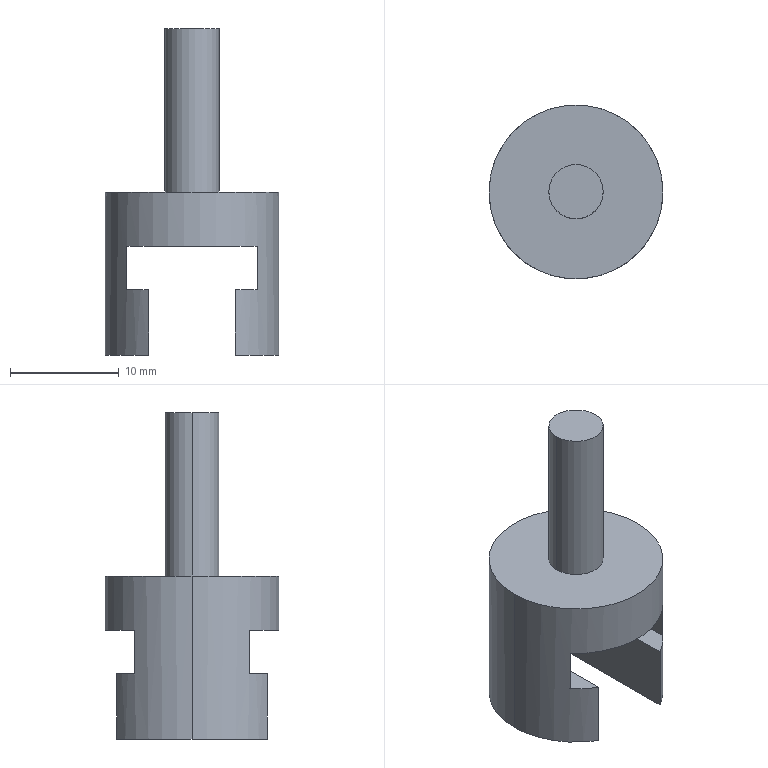Part | STEP file | 16 union | 1 solid | 15 faces | box 16 x 16 x 30 mm | volume 1888 mm3 | plane 11 | cylinder 4 | commonest cylinder face diameters 5 x2 16 x2
STEP:
#1=CARTESIAN_POINT('',(0.,0.,0.));
#2=DIRECTION('',(0.,0.,1.));
#3=DIRECTION('',(1.,0.,0.));
#4=AXIS2_PLACEMENT_3D('',#1,#2,#3);
#5=CARTESIAN_POINT('',(2.5,0.,30.));
#6=VERTEX_POINT('',#5);
#7=CARTESIAN_POINT('',(-2.5,0.,30.));
#8=VERTEX_POINT('',#7);
#9=CARTESIAN_POINT('',(0.,0.,30.));
#10=DIRECTION('',(0.,0.,1.));
#11=DIRECTION('',(1.,0.,0.));
#12=AXIS2_PLACEMENT_3D('',#9,#10,#11);
#13=CIRCLE('',#12,2.5);
#14=CARTESIAN_POINT('',(0.,0.,30.));
#15=DIRECTION('',(0.,0.,-1.));
#16=DIRECTION('',(-1.,0.,0.));
#17=AXIS2_PLACEMENT_3D('',#14,#15,#16);
#18=CYLINDRICAL_SURFACE('',#17,2.5);
#19=CARTESIAN_POINT('',(3.142,0.));
#20=DIRECTION('',(-1.,0.));
#21=VECTOR('',#20,1.);
#22=LINE('',#19,#21);
#23=(GEOMETRIC_REPRESENTATION_CONTEXT(2)PARAMETRIC_REPRESENTATION_CONTEXT()REPRESENTATION_CONTEXT('',''));
#24=DEFINITIONAL_REPRESENTATION('',(#22),#23);
#25=PCURVE('',#18,#24);
#26=CARTESIAN_POINT('',(0.,0.,30.));
#27=DIRECTION('',(0.,0.,1.));
#28=DIRECTION('',(1.,0.,0.));
#29=AXIS2_PLACEMENT_3D('',#26,#27,#28);
#30=PLANE('',#29);
#31=CARTESIAN_POINT('',(0.,0.));
#32=DIRECTION('',(1.,0.));
#33=AXIS2_PLACEMENT_2D('',#31,#32);
#34=CIRCLE('',#33,2.5);
#35=(GEOMETRIC_REPRESENTATION_CONTEXT(2)PARAMETRIC_REPRESENTATION_CONTEXT()REPRESENTATION_CONTEXT('',''));
#36=DEFINITIONAL_REPRESENTATION('',(#34),#35);
#37=PCURVE('',#30,#36);
#38=SURFACE_CURVE('',#13,(#25,#37),.PCURVE_S1.);
#39=EDGE_CURVE('',#6,#8,#38,.T.);
#40=ORIENTED_EDGE('',*,*,#39,.F.);
#41=CARTESIAN_POINT('',(2.5,0.,15.));
#42=VERTEX_POINT('',#41);
#43=CARTESIAN_POINT('',(2.5,0.,30.));
#44=DIRECTION('',(0.,0.,-1.));
#45=VECTOR('',#44,1.);
#46=LINE('',#43,#45);
#47=CARTESIAN_POINT('',(3.142,0.));
#48=DIRECTION('',(0.,1.));
#49=VECTOR('',#48,1.);
#50=LINE('',#47,#49);
#51=(GEOMETRIC_REPRESENTATION_CONTEXT(2)PARAMETRIC_REPRESENTATION_CONTEXT()REPRESENTATION_CONTEXT('',''));
#52=DEFINITIONAL_REPRESENTATION('',(#50),#51);
#53=PCURVE('',#18,#52);
#54=CARTESIAN_POINT('',(0.,0.,30.));
#55=DIRECTION('',(0.,0.,-1.));
#56=DIRECTION('',(-1.,0.,0.));
#57=AXIS2_PLACEMENT_3D('',#54,#55,#56);
#58=CYLINDRICAL_SURFACE('',#57,2.5);
#59=CARTESIAN_POINT('',(3.142,0.));
#60=DIRECTION('',(0.,1.));
#61=VECTOR('',#60,1.);
#62=LINE('',#59,#61);
#63=(GEOMETRIC_REPRESENTATION_CONTEXT(2)PARAMETRIC_REPRESENTATION_CONTEXT()REPRESENTATION_CONTEXT('',''));
#64=DEFINITIONAL_REPRESENTATION('',(#62),#63);
#65=PCURVE('',#58,#64);
#66=SURFACE_CURVE('',#46,(#53,#65),.PCURVE_S1.);
#67=EDGE_CURVE('',#6,#42,#66,.T.);
#68=ORIENTED_EDGE('',*,*,#67,.T.);
#69=CARTESIAN_POINT('',(-2.5,0.,15.));
#70=VERTEX_POINT('',#69);
#71=CARTESIAN_POINT('',(0.,0.,15.));
#72=DIRECTION('',(0.,0.,1.));
#73=DIRECTION('',(1.,0.,0.));
#74=AXIS2_PLACEMENT_3D('',#71,#72,#73);
#75=CIRCLE('',#74,2.5);
#76=CARTESIAN_POINT('',(3.142,15.));
#77=DIRECTION('',(-1.,0.));
#78=VECTOR('',#77,1.);
#79=LINE('',#76,#78);
#80=(GEOMETRIC_REPRESENTATION_CONTEXT(2)PARAMETRIC_REPRESENTATION_CONTEXT()REPRESENTATION_CONTEXT('',''));
#81=DEFINITIONAL_REPRESENTATION('',(#79),#80);
#82=PCURVE('',#18,#81);
#83=CARTESIAN_POINT('',(0.,0.,15.));
#84=DIRECTION('',(0.,0.,1.));
#85=DIRECTION('',(1.,0.,0.));
#86=AXIS2_PLACEMENT_3D('',#83,#84,#85);
#87=PLANE('',#86);
#88=CARTESIAN_POINT('',(0.,0.));
#89=DIRECTION('',(1.,0.));
#90=AXIS2_PLACEMENT_2D('',#88,#89);
#91=CIRCLE('',#90,2.5);
#92=(GEOMETRIC_REPRESENTATION_CONTEXT(2)PARAMETRIC_REPRESENTATION_CONTEXT()REPRESENTATION_CONTEXT('',''));
#93=DEFINITIONAL_REPRESENTATION('',(#91),#92);
#94=PCURVE('',#87,#93);
#95=SURFACE_CURVE('',#75,(#82,#94),.PCURVE_S1.);
#96=EDGE_CURVE('',#42,#70,#95,.T.);
#97=ORIENTED_EDGE('',*,*,#96,.T.);
#98=CARTESIAN_POINT('',(-2.5,0.,30.));
#99=DIRECTION('',(0.,0.,-1.));
#100=VECTOR('',#99,1.);
#101=LINE('',#98,#100);
#102=CARTESIAN_POINT('',(0.,0.));
#103=DIRECTION('',(0.,1.));
#104=VECTOR('',#103,1.);
#105=LINE('',#102,#104);
#106=(GEOMETRIC_REPRESENTATION_CONTEXT(2)PARAMETRIC_REPRESENTATION_CONTEXT()REPRESENTATION_CONTEXT('',''));
#107=DEFINITIONAL_REPRESENTATION('',(#105),#106);
#108=PCURVE('',#18,#107);
#109=CARTESIAN_POINT('',(6.283,0.));
#110=DIRECTION('',(0.,1.));
#111=VECTOR('',#110,1.);
#112=LINE('',#109,#111);
#113=(GEOMETRIC_REPRESENTATION_CONTEXT(2)PARAMETRIC_REPRESENTATION_CONTEXT()REPRESENTATION_CONTEXT('',''));
#114=DEFINITIONAL_REPRESENTATION('',(#112),#113);
#115=PCURVE('',#58,#114);
#116=SURFACE_CURVE('',#101,(#108,#115),.PCURVE_S1.);
#117=EDGE_CURVE('',#8,#70,#116,.T.);
#118=ORIENTED_EDGE('',*,*,#117,.F.);
#119=EDGE_LOOP('',(#40,#68,#97,#118));
#120=FACE_BOUND('',#119,.T.);
#121=ADVANCED_FACE('',(#120),#18,.T.);
#122=CARTESIAN_POINT('',(8.,0.,15.));
#123=VERTEX_POINT('',#122);
#124=CARTESIAN_POINT('',(-8.,0.,15.));
#125=VERTEX_POINT('',#124);
#126=CARTESIAN_POINT('',(0.,0.,15.));
#127=DIRECTION('',(0.,0.,1.));
#128=DIRECTION('',(1.,0.,0.));
#129=AXIS2_PLACEMENT_3D('',#126,#127,#128);
#130=CIRCLE('',#129,8.);
#131=CARTESIAN_POINT('',(0.,0.,15.));
#132=DIRECTION('',(0.,0.,-1.));
#133=DIRECTION('',(-1.,0.,0.));
#134=AXIS2_PLACEMENT_3D('',#131,#132,#133);
#135=CYLINDRICAL_SURFACE('',#134,8.);
#136=CARTESIAN_POINT('',(3.142,0.));
#137=DIRECTION('',(-1.,0.));
#138=VECTOR('',#137,1.);
#139=LINE('',#136,#138);
#140=(GEOMETRIC_REPRESENTATION_CONTEXT(2)PARAMETRIC_REPRESENTATION_CONTEXT()REPRESENTATION_CONTEXT('',''));
#141=DEFINITIONAL_REPRESENTATION('',(#139),#140);
#142=PCURVE('',#135,#141);
#143=CARTESIAN_POINT('',(0.,0.));
#144=DIRECTION('',(1.,0.));
#145=AXIS2_PLACEMENT_2D('',#143,#144);
#146=CIRCLE('',#145,8.);
#147=(GEOMETRIC_REPRESENTATION_CONTEXT(2)PARAMETRIC_REPRESENTATION_CONTEXT()REPRESENTATION_CONTEXT('',''));
#148=DEFINITIONAL_REPRESENTATION('',(#146),#147);
#149=PCURVE('',#87,#148);
#150=SURFACE_CURVE('',#130,(#142,#149),.PCURVE_S1.);
#151=EDGE_CURVE('',#123,#125,#150,.T.);
#152=ORIENTED_EDGE('',*,*,#151,.F.);
#153=CARTESIAN_POINT('',(8.,0.,0.));
#154=VERTEX_POINT('',#153);
#155=CARTESIAN_POINT('',(8.,0.,15.));
#156=DIRECTION('',(0.,0.,-1.));
#157=VECTOR('',#156,1.);
#158=LINE('',#155,#157);
#159=CARTESIAN_POINT('',(3.142,0.));
#160=DIRECTION('',(0.,1.));
#161=VECTOR('',#160,1.);
#162=LINE('',#159,#161);
#163=(GEOMETRIC_REPRESENTATION_CONTEXT(2)PARAMETRIC_REPRESENTATION_CONTEXT()REPRESENTATION_CONTEXT('',''));
#164=DEFINITIONAL_REPRESENTATION('',(#162),#163);
#165=PCURVE('',#135,#164);
#166=CARTESIAN_POINT('',(0.,0.,15.));
#167=DIRECTION('',(0.,0.,-1.));
#168=DIRECTION('',(-1.,0.,0.));
#169=AXIS2_PLACEMENT_3D('',#166,#167,#168);
#170=CYLINDRICAL_SURFACE('',#169,8.);
#171=CARTESIAN_POINT('',(3.142,0.));
#172=DIRECTION('',(0.,1.));
#173=VECTOR('',#172,1.);
#174=LINE('',#171,#173);
#175=(GEOMETRIC_REPRESENTATION_CONTEXT(2)PARAMETRIC_REPRESENTATION_CONTEXT()REPRESENTATION_CONTEXT('',''));
#176=DEFINITIONAL_REPRESENTATION('',(#174),#175);
#177=PCURVE('',#170,#176);
#178=SURFACE_CURVE('',#158,(#165,#177),.PCURVE_S1.);
#179=EDGE_CURVE('',#123,#154,#178,.T.);
#180=ORIENTED_EDGE('',*,*,#179,.T.);
#181=CARTESIAN_POINT('',(4.,6.928,0.));
#182=VERTEX_POINT('',#181);
#183=CARTESIAN_POINT('',(0.,0.,0.));
#184=DIRECTION('',(0.,0.,1.));
#185=DIRECTION('',(1.,0.,0.));
#186=AXIS2_PLACEMENT_3D('',#183,#184,#185);
#187=CIRCLE('',#186,8.);
#188=CARTESIAN_POINT('',(3.142,15.));
#189=DIRECTION('',(-1.,0.));
#190=VECTOR('',#189,1.);
#191=LINE('',#188,#190);
#192=(GEOMETRIC_REPRESENTATION_CONTEXT(2)PARAMETRIC_REPRESENTATION_CONTEXT()REPRESENTATION_CONTEXT('',''));
#193=DEFINITIONAL_REPRESENTATION('',(#191),#192);
#194=PCURVE('',#135,#193);
#195=CARTESIAN_POINT('',(0.,0.,0.));
#196=DIRECTION('',(0.,0.,1.));
#197=DIRECTION('',(1.,0.,0.));
#198=AXIS2_PLACEMENT_3D('',#195,#196,#197);
#199=PLANE('',#198);
#200=CARTESIAN_POINT('',(0.,0.));
#201=DIRECTION('',(1.,0.));
#202=AXIS2_PLACEMENT_2D('',#200,#201);
#203=CIRCLE('',#202,8.);
#204=(GEOMETRIC_REPRESENTATION_CONTEXT(2)PARAMETRIC_REPRESENTATION_CONTEXT()REPRESENTATION_CONTEXT('',''));
#205=DEFINITIONAL_REPRESENTATION('',(#203),#204);
#206=PCURVE('',#199,#205);
#207=SURFACE_CURVE('',#187,(#194,#206),.PCURVE_S1.);
#208=EDGE_CURVE('',#154,#182,#207,.T.);
#209=ORIENTED_EDGE('',*,*,#208,.T.);
#210=CARTESIAN_POINT('',(4.,6.928,6.));
#211=VERTEX_POINT('',#210);
#212=CARTESIAN_POINT('',(4.,6.928,15.));
#213=DIRECTION('',(0.,0.,-1.));
#214=VECTOR('',#213,1.);
#215=LINE('',#212,#214);
#216=CARTESIAN_POINT('',(2.094,0.));
#217=DIRECTION('',(0.,1.));
#218=VECTOR('',#217,1.);
#219=LINE('',#216,#218);
#220=(GEOMETRIC_REPRESENTATION_CONTEXT(2)PARAMETRIC_REPRESENTATION_CONTEXT()REPRESENTATION_CONTEXT('',''));
#221=DEFINITIONAL_REPRESENTATION('',(#219),#220);
#222=PCURVE('',#135,#221);
#223=CARTESIAN_POINT('',(4.,10.,6.));
#224=DIRECTION('',(-1.,0.,0.));
#225=DIRECTION('',(0.,0.,1.));
#226=AXIS2_PLACEMENT_3D('',#223,#224,#225);
#227=PLANE('',#226);
#228=CARTESIAN_POINT('',(9.,-3.072));
#229=DIRECTION('',(-1.,0.));
#230=VECTOR('',#229,1.);
#231=LINE('',#228,#230);
#232=(GEOMETRIC_REPRESENTATION_CONTEXT(2)PARAMETRIC_REPRESENTATION_CONTEXT()REPRESENTATION_CONTEXT('',''));
#233=DEFINITIONAL_REPRESENTATION('',(#231),#232);
#234=PCURVE('',#227,#233);
#235=SURFACE_CURVE('',#215,(#222,#234),.PCURVE_S1.);
#236=EDGE_CURVE('',#211,#182,#235,.T.);
#237=ORIENTED_EDGE('',*,*,#236,.F.);
#238=CARTESIAN_POINT('',(6.,5.292,6.));
#239=VERTEX_POINT('',#238);
#240=CARTESIAN_POINT('',(0.,0.,6.));
#241=DIRECTION('',(0.,0.,1.));
#242=DIRECTION('',(1.,0.,0.));
#243=AXIS2_PLACEMENT_3D('',#240,#241,#242);
#244=CIRCLE('',#243,8.);
#245=CARTESIAN_POINT('',(3.142,9.));
#246=DIRECTION('',(-1.,0.));
#247=VECTOR('',#246,1.);
#248=LINE('',#245,#247);
#249=(GEOMETRIC_REPRESENTATION_CONTEXT(2)PARAMETRIC_REPRESENTATION_CONTEXT()REPRESENTATION_CONTEXT('',''));
#250=DEFINITIONAL_REPRESENTATION('',(#248),#249);
#251=PCURVE('',#135,#250);
#252=CARTESIAN_POINT('',(6.,10.,6.));
#253=DIRECTION('',(0.,0.,1.));
#254=DIRECTION('',(1.,0.,0.));
#255=AXIS2_PLACEMENT_3D('',#252,#253,#254);
#256=PLANE('',#255);
#257=CARTESIAN_POINT('',(-6.,-10.));
#258=DIRECTION('',(1.,0.));
#259=AXIS2_PLACEMENT_2D('',#257,#258);
#260=CIRCLE('',#259,8.);
#261=(GEOMETRIC_REPRESENTATION_CONTEXT(2)PARAMETRIC_REPRESENTATION_CONTEXT()REPRESENTATION_CONTEXT('',''));
#262=DEFINITIONAL_REPRESENTATION('',(#260),#261);
#263=PCURVE('',#256,#262);
#264=SURFACE_CURVE('',#244,(#251,#263),.PCURVE_S1.);
#265=EDGE_CURVE('',#239,#211,#264,.T.);
#266=ORIENTED_EDGE('',*,*,#265,.F.);
#267=CARTESIAN_POINT('',(6.,5.292,10.));
#268=VERTEX_POINT('',#267);
#269=CARTESIAN_POINT('',(6.,5.292,15.));
#270=DIRECTION('',(0.,0.,-1.));
#271=VECTOR('',#270,1.);
#272=LINE('',#269,#271);
#273=CARTESIAN_POINT('',(2.419,0.));
#274=DIRECTION('',(0.,1.));
#275=VECTOR('',#274,1.);
#276=LINE('',#273,#275);
#277=(GEOMETRIC_REPRESENTATION_CONTEXT(2)PARAMETRIC_REPRESENTATION_CONTEXT()REPRESENTATION_CONTEXT('',''));
#278=DEFINITIONAL_REPRESENTATION('',(#276),#277);
#279=PCURVE('',#135,#278);
#280=CARTESIAN_POINT('',(6.,10.,10.));
#281=DIRECTION('',(-1.,0.,0.));
#282=DIRECTION('',(0.,0.,1.));
#283=AXIS2_PLACEMENT_3D('',#280,#281,#282);
#284=PLANE('',#283);
#285=CARTESIAN_POINT('',(5.,-4.708));
#286=DIRECTION('',(-1.,0.));
#287=VECTOR('',#286,1.);
#288=LINE('',#285,#287);
#289=(GEOMETRIC_REPRESENTATION_CONTEXT(2)PARAMETRIC_REPRESENTATION_CONTEXT()REPRESENTATION_CONTEXT('',''));
#290=DEFINITIONAL_REPRESENTATION('',(#288),#289);
#291=PCURVE('',#284,#290);
#292=SURFACE_CURVE('',#272,(#279,#291),.PCURVE_S1.);
#293=EDGE_CURVE('',#268,#239,#292,.T.);
#294=ORIENTED_EDGE('',*,*,#293,.F.);
#295=CARTESIAN_POINT('',(-6.,5.292,10.));
#296=VERTEX_POINT('',#295);
#297=CARTESIAN_POINT('',(0.,0.,10.));
#298=DIRECTION('',(0.,0.,-1.));
#299=DIRECTION('',(-1.,0.,0.));
#300=AXIS2_PLACEMENT_3D('',#297,#298,#299);
#301=CIRCLE('',#300,8.);
#302=CARTESIAN_POINT('',(0.,5.));
#303=DIRECTION('',(1.,0.));
#304=VECTOR('',#303,1.);
#305=LINE('',#302,#304);
#306=(GEOMETRIC_REPRESENTATION_CONTEXT(2)PARAMETRIC_REPRESENTATION_CONTEXT()REPRESENTATION_CONTEXT('',''));
#307=DEFINITIONAL_REPRESENTATION('',(#305),#306);
#308=PCURVE('',#135,#307);
#309=CARTESIAN_POINT('',(6.,10.,10.));
#310=DIRECTION('',(0.,0.,-1.));
#311=DIRECTION('',(-1.,0.,0.));
#312=AXIS2_PLACEMENT_3D('',#309,#310,#311);
#313=PLANE('',#312);
#314=CARTESIAN_POINT('',(6.,-10.));
#315=DIRECTION('',(1.,0.));
#316=AXIS2_PLACEMENT_2D('',#314,#315);
#317=CIRCLE('',#316,8.);
#318=(GEOMETRIC_REPRESENTATION_CONTEXT(2)PARAMETRIC_REPRESENTATION_CONTEXT()REPRESENTATION_CONTEXT('',''));
#319=DEFINITIONAL_REPRESENTATION('',(#317),#318);
#320=PCURVE('',#313,#319);
#321=SURFACE_CURVE('',#301,(#308,#320),.PCURVE_S1.);
#322=EDGE_CURVE('',#296,#268,#321,.T.);
#323=ORIENTED_EDGE('',*,*,#322,.F.);
#324=CARTESIAN_POINT('',(-6.,5.292,6.));
#325=VERTEX_POINT('',#324);
#326=CARTESIAN_POINT('',(-6.,5.292,15.));
#327=DIRECTION('',(0.,0.,1.));
#328=VECTOR('',#327,1.);
#329=LINE('',#326,#328);
#330=CARTESIAN_POINT('',(0.7227,0.));
#331=DIRECTION('',(0.,-1.));
#332=VECTOR('',#331,1.);
#333=LINE('',#330,#332);
#334=(GEOMETRIC_REPRESENTATION_CONTEXT(2)PARAMETRIC_REPRESENTATION_CONTEXT()REPRESENTATION_CONTEXT('',''));
#335=DEFINITIONAL_REPRESENTATION('',(#333),#334);
#336=PCURVE('',#135,#335);
#337=CARTESIAN_POINT('',(-6.,10.,10.));
#338=DIRECTION('',(1.,0.,0.));
#339=DIRECTION('',(0.,0.,-1.));
#340=AXIS2_PLACEMENT_3D('',#337,#338,#339);
#341=PLANE('',#340);
#342=CARTESIAN_POINT('',(-5.,-4.708));
#343=DIRECTION('',(-1.,0.));
#344=VECTOR('',#343,1.);
#345=LINE('',#342,#344);
#346=(GEOMETRIC_REPRESENTATION_CONTEXT(2)PARAMETRIC_REPRESENTATION_CONTEXT()REPRESENTATION_CONTEXT('',''));
#347=DEFINITIONAL_REPRESENTATION('',(#345),#346);
#348=PCURVE('',#341,#347);
#349=SURFACE_CURVE('',#329,(#336,#348),.PCURVE_S1.);
#350=EDGE_CURVE('',#325,#296,#349,.T.);
#351=ORIENTED_EDGE('',*,*,#350,.F.);
#352=CARTESIAN_POINT('',(-4.,6.928,6.));
#353=VERTEX_POINT('',#352);
#354=CARTESIAN_POINT('',(0.,0.,6.));
#355=DIRECTION('',(0.,0.,1.));
#356=DIRECTION('',(1.,0.,0.));
#357=AXIS2_PLACEMENT_3D('',#354,#355,#356);
#358=CIRCLE('',#357,8.);
#359=CARTESIAN_POINT('',(3.142,9.));
#360=DIRECTION('',(-1.,0.));
#361=VECTOR('',#360,1.);
#362=LINE('',#359,#361);
#363=(GEOMETRIC_REPRESENTATION_CONTEXT(2)PARAMETRIC_REPRESENTATION_CONTEXT()REPRESENTATION_CONTEXT('',''));
#364=DEFINITIONAL_REPRESENTATION('',(#362),#363);
#365=PCURVE('',#135,#364);
#366=CARTESIAN_POINT('',(-6.,10.,6.));
#367=DIRECTION('',(0.,0.,1.));
#368=DIRECTION('',(1.,0.,0.));
#369=AXIS2_PLACEMENT_3D('',#366,#367,#368);
#370=PLANE('',#369);
#371=CARTESIAN_POINT('',(6.,-10.));
#372=DIRECTION('',(1.,0.));
#373=AXIS2_PLACEMENT_2D('',#371,#372);
#374=CIRCLE('',#373,8.);
#375=(GEOMETRIC_REPRESENTATION_CONTEXT(2)PARAMETRIC_REPRESENTATION_CONTEXT()REPRESENTATION_CONTEXT('',''));
#376=DEFINITIONAL_REPRESENTATION('',(#374),#375);
#377=PCURVE('',#370,#376);
#378=SURFACE_CURVE('',#358,(#365,#377),.PCURVE_S1.);
#379=EDGE_CURVE('',#353,#325,#378,.T.);
#380=ORIENTED_EDGE('',*,*,#379,.F.);
#381=CARTESIAN_POINT('',(-4.,6.928,0.));
#382=VERTEX_POINT('',#381);
#383=CARTESIAN_POINT('',(-4.,6.928,15.));
#384=DIRECTION('',(0.,0.,1.));
#385=VECTOR('',#384,1.);
#386=LINE('',#383,#385);
#387=CARTESIAN_POINT('',(1.047,0.));
#388=DIRECTION('',(0.,-1.));
#389=VECTOR('',#388,1.);
#390=LINE('',#387,#389);
#391=(GEOMETRIC_REPRESENTATION_CONTEXT(2)PARAMETRIC_REPRESENTATION_CONTEXT()REPRESENTATION_CONTEXT('',''));
#392=DEFINITIONAL_REPRESENTATION('',(#390),#391);
#393=PCURVE('',#135,#392);
#394=CARTESIAN_POINT('',(-4.,10.,6.));
#395=DIRECTION('',(1.,0.,0.));
#396=DIRECTION('',(0.,0.,-1.));
#397=AXIS2_PLACEMENT_3D('',#394,#395,#396);
#398=PLANE('',#397);
#399=CARTESIAN_POINT('',(-9.,-3.072));
#400=DIRECTION('',(-1.,0.));
#401=VECTOR('',#400,1.);
#402=LINE('',#399,#401);
#403=(GEOMETRIC_REPRESENTATION_CONTEXT(2)PARAMETRIC_REPRESENTATION_CONTEXT()REPRESENTATION_CONTEXT('',''));
#404=DEFINITIONAL_REPRESENTATION('',(#402),#403);
#405=PCURVE('',#398,#404);
#406=SURFACE_CURVE('',#386,(#393,#405),.PCURVE_S1.);
#407=EDGE_CURVE('',#382,#353,#406,.T.);
#408=ORIENTED_EDGE('',*,*,#407,.F.);
#409=CARTESIAN_POINT('',(-8.,0.,0.));
#410=VERTEX_POINT('',#409);
#411=CARTESIAN_POINT('',(0.,0.,0.));
#412=DIRECTION('',(0.,0.,1.));
#413=DIRECTION('',(1.,0.,0.));
#414=AXIS2_PLACEMENT_3D('',#411,#412,#413);
#415=CIRCLE('',#414,8.);
#416=CARTESIAN_POINT('',(3.142,15.));
#417=DIRECTION('',(-1.,0.));
#418=VECTOR('',#417,1.);
#419=LINE('',#416,#418);
#420=(GEOMETRIC_REPRESENTATION_CONTEXT(2)PARAMETRIC_REPRESENTATION_CONTEXT()REPRESENTATION_CONTEXT('',''));
#421=DEFINITIONAL_REPRESENTATION('',(#419),#420);
#422=PCURVE('',#135,#421);
#423=CARTESIAN_POINT('',(0.,0.,0.));
#424=DIRECTION('',(0.,0.,1.));
#425=DIRECTION('',(1.,0.,0.));
#426=AXIS2_PLACEMENT_3D('',#423,#424,#425);
#427=PLANE('',#426);
#428=CARTESIAN_POINT('',(0.,0.));
#429=DIRECTION('',(1.,0.));
#430=AXIS2_PLACEMENT_2D('',#428,#429);
#431=CIRCLE('',#430,8.);
#432=(GEOMETRIC_REPRESENTATION_CONTEXT(2)PARAMETRIC_REPRESENTATION_CONTEXT()REPRESENTATION_CONTEXT('',''));
#433=DEFINITIONAL_REPRESENTATION('',(#431),#432);
#434=PCURVE('',#427,#433);
#435=SURFACE_CURVE('',#415,(#422,#434),.PCURVE_S1.);
#436=EDGE_CURVE('',#382,#410,#435,.T.);
#437=ORIENTED_EDGE('',*,*,#436,.T.);
#438=CARTESIAN_POINT('',(-8.,0.,15.));
#439=DIRECTION('',(0.,0.,-1.));
#440=VECTOR('',#439,1.);
#441=LINE('',#438,#440);
#442=CARTESIAN_POINT('',(0.,0.));
#443=DIRECTION('',(0.,1.));
#444=VECTOR('',#443,1.);
#445=LINE('',#442,#444);
#446=(GEOMETRIC_REPRESENTATION_CONTEXT(2)PARAMETRIC_REPRESENTATION_CONTEXT()REPRESENTATION_CONTEXT('',''));
#447=DEFINITIONAL_REPRESENTATION('',(#445),#446);
#448=PCURVE('',#135,#447);
#449=CARTESIAN_POINT('',(6.283,0.));
#450=DIRECTION('',(0.,1.));
#451=VECTOR('',#450,1.);
#452=LINE('',#449,#451);
#453=(GEOMETRIC_REPRESENTATION_CONTEXT(2)PARAMETRIC_REPRESENTATION_CONTEXT()REPRESENTATION_CONTEXT('',''));
#454=DEFINITIONAL_REPRESENTATION('',(#452),#453);
#455=PCURVE('',#170,#454);
#456=SURFACE_CURVE('',#441,(#448,#455),.PCURVE_S1.);
#457=EDGE_CURVE('',#125,#410,#456,.T.);
#458=ORIENTED_EDGE('',*,*,#457,.F.);
#459=EDGE_LOOP('',(#152,#180,#209,#237,#266,#294,#323,#351,#380,#408,#437,#458));
#460=FACE_BOUND('',#459,.T.);
#461=ADVANCED_FACE('',(#460),#135,.T.);
#462=CARTESIAN_POINT('',(0.,0.,15.));
#463=DIRECTION('',(0.,0.,1.));
#464=DIRECTION('',(1.,0.,0.));
#465=AXIS2_PLACEMENT_3D('',#462,#463,#464);
#466=CIRCLE('',#465,8.);
#467=CARTESIAN_POINT('',(0.,0.));
#468=DIRECTION('',(1.,0.));
#469=AXIS2_PLACEMENT_2D('',#467,#468);
#470=CIRCLE('',#469,8.);
#471=(GEOMETRIC_REPRESENTATION_CONTEXT(2)PARAMETRIC_REPRESENTATION_CONTEXT()REPRESENTATION_CONTEXT('',''));
#472=DEFINITIONAL_REPRESENTATION('',(#470),#471);
#473=PCURVE('',#87,#472);
#474=CARTESIAN_POINT('',(9.425,0.));
#475=DIRECTION('',(-1.,0.));
#476=VECTOR('',#475,1.);
#477=LINE('',#474,#476);
#478=(GEOMETRIC_REPRESENTATION_CONTEXT(2)PARAMETRIC_REPRESENTATION_CONTEXT()REPRESENTATION_CONTEXT('',''));
#479=DEFINITIONAL_REPRESENTATION('',(#477),#478);
#480=PCURVE('',#170,#479);
#481=SURFACE_CURVE('',#466,(#473,#480),.PCURVE_S1.);
#482=EDGE_CURVE('',#125,#123,#481,.T.);
#483=ORIENTED_EDGE('',*,*,#482,.T.);
#484=ORIENTED_EDGE('',*,*,#151,.T.);
#485=EDGE_LOOP('',(#483,#484));
#486=FACE_BOUND('',#485,.T.);
#487=CARTESIAN_POINT('',(0.,0.,15.));
#488=DIRECTION('',(0.,0.,1.));
#489=DIRECTION('',(1.,0.,0.));
#490=AXIS2_PLACEMENT_3D('',#487,#488,#489);
#491=CIRCLE('',#490,2.5);
#492=CARTESIAN_POINT('',(0.,0.));
#493=DIRECTION('',(1.,0.));
#494=AXIS2_PLACEMENT_2D('',#492,#493);
#495=CIRCLE('',#494,2.5);
#496=(GEOMETRIC_REPRESENTATION_CONTEXT(2)PARAMETRIC_REPRESENTATION_CONTEXT()REPRESENTATION_CONTEXT('',''));
#497=DEFINITIONAL_REPRESENTATION('',(#495),#496);
#498=PCURVE('',#87,#497);
#499=CARTESIAN_POINT('',(9.425,15.));
#500=DIRECTION('',(-1.,0.));
#501=VECTOR('',#500,1.);
#502=LINE('',#499,#501);
#503=(GEOMETRIC_REPRESENTATION_CONTEXT(2)PARAMETRIC_REPRESENTATION_CONTEXT()REPRESENTATION_CONTEXT('',''));
#504=DEFINITIONAL_REPRESENTATION('',(#502),#503);
#505=PCURVE('',#58,#504);
#506=SURFACE_CURVE('',#491,(#498,#505),.PCURVE_S1.);
#507=EDGE_CURVE('',#70,#42,#506,.T.);
#508=ORIENTED_EDGE('',*,*,#507,.F.);
#509=ORIENTED_EDGE('',*,*,#96,.F.);
#510=EDGE_LOOP('',(#508,#509));
#511=FACE_BOUND('',#510,.T.);
#512=ADVANCED_FACE('',(#486,#511),#87,.T.);
#513=ORIENTED_EDGE('',*,*,#179,.F.);
#514=ORIENTED_EDGE('',*,*,#482,.F.);
#515=ORIENTED_EDGE('',*,*,#457,.T.);
#516=CARTESIAN_POINT('',(-4.,-6.928,0.));
#517=VERTEX_POINT('',#516);
#518=CARTESIAN_POINT('',(0.,0.,0.));
#519=DIRECTION('',(0.,0.,1.));
#520=DIRECTION('',(1.,0.,0.));
#521=AXIS2_PLACEMENT_3D('',#518,#519,#520);
#522=CIRCLE('',#521,8.);
#523=CARTESIAN_POINT('',(9.425,15.));
#524=DIRECTION('',(-1.,0.));
#525=VECTOR('',#524,1.);
#526=LINE('',#523,#525);
#527=(GEOMETRIC_REPRESENTATION_CONTEXT(2)PARAMETRIC_REPRESENTATION_CONTEXT()REPRESENTATION_CONTEXT('',''));
#528=DEFINITIONAL_REPRESENTATION('',(#526),#527);
#529=PCURVE('',#170,#528);
#530=CARTESIAN_POINT('',(0.,0.));
#531=DIRECTION('',(1.,0.));
#532=AXIS2_PLACEMENT_2D('',#530,#531);
#533=CIRCLE('',#532,8.);
#534=(GEOMETRIC_REPRESENTATION_CONTEXT(2)PARAMETRIC_REPRESENTATION_CONTEXT()REPRESENTATION_CONTEXT('',''));
#535=DEFINITIONAL_REPRESENTATION('',(#533),#534);
#536=PCURVE('',#427,#535);
#537=SURFACE_CURVE('',#522,(#529,#536),.PCURVE_S1.);
#538=EDGE_CURVE('',#410,#517,#537,.T.);
#539=ORIENTED_EDGE('',*,*,#538,.T.);
#540=CARTESIAN_POINT('',(-4.,-6.928,6.));
#541=VERTEX_POINT('',#540);
#542=CARTESIAN_POINT('',(-4.,-6.928,15.));
#543=DIRECTION('',(0.,0.,-1.));
#544=VECTOR('',#543,1.);
#545=LINE('',#542,#544);
#546=CARTESIAN_POINT('',(5.236,0.));
#547=DIRECTION('',(0.,1.));
#548=VECTOR('',#547,1.);
#549=LINE('',#546,#548);
#550=(GEOMETRIC_REPRESENTATION_CONTEXT(2)PARAMETRIC_REPRESENTATION_CONTEXT()REPRESENTATION_CONTEXT('',''));
#551=DEFINITIONAL_REPRESENTATION('',(#549),#550);
#552=PCURVE('',#170,#551);
#553=CARTESIAN_POINT('',(-9.,-16.928));
#554=DIRECTION('',(1.,0.));
#555=VECTOR('',#554,1.);
#556=LINE('',#553,#555);
#557=(GEOMETRIC_REPRESENTATION_CONTEXT(2)PARAMETRIC_REPRESENTATION_CONTEXT()REPRESENTATION_CONTEXT('',''));
#558=DEFINITIONAL_REPRESENTATION('',(#556),#557);
#559=PCURVE('',#398,#558);
#560=SURFACE_CURVE('',#545,(#552,#559),.PCURVE_S1.);
#561=EDGE_CURVE('',#541,#517,#560,.T.);
#562=ORIENTED_EDGE('',*,*,#561,.F.);
#563=CARTESIAN_POINT('',(-6.,-5.292,6.));
#564=VERTEX_POINT('',#563);
#565=CARTESIAN_POINT('',(0.,0.,6.));
#566=DIRECTION('',(0.,0.,1.));
#567=DIRECTION('',(1.,0.,0.));
#568=AXIS2_PLACEMENT_3D('',#565,#566,#567);
#569=CIRCLE('',#568,8.);
#570=CARTESIAN_POINT('',(9.425,9.));
#571=DIRECTION('',(-1.,0.));
#572=VECTOR('',#571,1.);
#573=LINE('',#570,#572);
#574=(GEOMETRIC_REPRESENTATION_CONTEXT(2)PARAMETRIC_REPRESENTATION_CONTEXT()REPRESENTATION_CONTEXT('',''));
#575=DEFINITIONAL_REPRESENTATION('',(#573),#574);
#576=PCURVE('',#170,#575);
#577=CARTESIAN_POINT('',(6.,-10.));
#578=DIRECTION('',(1.,0.));
#579=AXIS2_PLACEMENT_2D('',#577,#578);
#580=CIRCLE('',#579,8.);
#581=(GEOMETRIC_REPRESENTATION_CONTEXT(2)PARAMETRIC_REPRESENTATION_CONTEXT()REPRESENTATION_CONTEXT('',''));
#582=DEFINITIONAL_REPRESENTATION('',(#580),#581);
#583=PCURVE('',#370,#582);
#584=SURFACE_CURVE('',#569,(#576,#583),.PCURVE_S1.);
#585=EDGE_CURVE('',#564,#541,#584,.T.);
#586=ORIENTED_EDGE('',*,*,#585,.F.);
#587=CARTESIAN_POINT('',(-6.,-5.292,10.));
#588=VERTEX_POINT('',#587);
#589=CARTESIAN_POINT('',(-6.,-5.292,15.));
#590=DIRECTION('',(0.,0.,-1.));
#591=VECTOR('',#590,1.);
#592=LINE('',#589,#591);
#593=CARTESIAN_POINT('',(5.56,0.));
#594=DIRECTION('',(0.,1.));
#595=VECTOR('',#594,1.);
#596=LINE('',#593,#595);
#597=(GEOMETRIC_REPRESENTATION_CONTEXT(2)PARAMETRIC_REPRESENTATION_CONTEXT()REPRESENTATION_CONTEXT('',''));
#598=DEFINITIONAL_REPRESENTATION('',(#596),#597);
#599=PCURVE('',#170,#598);
#600=CARTESIAN_POINT('',(-5.,-15.292));
#601=DIRECTION('',(1.,0.));
#602=VECTOR('',#601,1.);
#603=LINE('',#600,#602);
#604=(GEOMETRIC_REPRESENTATION_CONTEXT(2)PARAMETRIC_REPRESENTATION_CONTEXT()REPRESENTATION_CONTEXT('',''));
#605=DEFINITIONAL_REPRESENTATION('',(#603),#604);
#606=PCURVE('',#341,#605);
#607=SURFACE_CURVE('',#592,(#599,#606),.PCURVE_S1.);
#608=EDGE_CURVE('',#588,#564,#607,.T.);
#609=ORIENTED_EDGE('',*,*,#608,.F.);
#610=CARTESIAN_POINT('',(6.,-5.292,10.));
#611=VERTEX_POINT('',#610);
#612=CARTESIAN_POINT('',(0.,0.,10.));
#613=DIRECTION('',(0.,0.,-1.));
#614=DIRECTION('',(-1.,0.,0.));
#615=AXIS2_PLACEMENT_3D('',#612,#613,#614);
#616=CIRCLE('',#615,8.);
#617=CARTESIAN_POINT('',(0.,5.));
#618=DIRECTION('',(1.,0.));
#619=VECTOR('',#618,1.);
#620=LINE('',#617,#619);
#621=(GEOMETRIC_REPRESENTATION_CONTEXT(2)PARAMETRIC_REPRESENTATION_CONTEXT()REPRESENTATION_CONTEXT('',''));
#622=DEFINITIONAL_REPRESENTATION('',(#620),#621);
#623=PCURVE('',#170,#622);
#624=CARTESIAN_POINT('',(6.,-10.));
#625=DIRECTION('',(1.,0.));
#626=AXIS2_PLACEMENT_2D('',#624,#625);
#627=CIRCLE('',#626,8.);
#628=(GEOMETRIC_REPRESENTATION_CONTEXT(2)PARAMETRIC_REPRESENTATION_CONTEXT()REPRESENTATION_CONTEXT('',''));
#629=DEFINITIONAL_REPRESENTATION('',(#627),#628);
#630=PCURVE('',#313,#629);
#631=SURFACE_CURVE('',#616,(#623,#630),.PCURVE_S1.);
#632=EDGE_CURVE('',#611,#588,#631,.T.);
#633=ORIENTED_EDGE('',*,*,#632,.F.);
#634=CARTESIAN_POINT('',(6.,-5.292,6.));
#635=VERTEX_POINT('',#634);
#636=CARTESIAN_POINT('',(6.,-5.292,15.));
#637=DIRECTION('',(0.,0.,1.));
#638=VECTOR('',#637,1.);
#639=LINE('',#636,#638);
#640=CARTESIAN_POINT('',(3.864,0.));
#641=DIRECTION('',(0.,-1.));
#642=VECTOR('',#641,1.);
#643=LINE('',#640,#642);
#644=(GEOMETRIC_REPRESENTATION_CONTEXT(2)PARAMETRIC_REPRESENTATION_CONTEXT()REPRESENTATION_CONTEXT('',''));
#645=DEFINITIONAL_REPRESENTATION('',(#643),#644);
#646=PCURVE('',#170,#645);
#647=CARTESIAN_POINT('',(5.,-15.292));
#648=DIRECTION('',(1.,0.));
#649=VECTOR('',#648,1.);
#650=LINE('',#647,#649);
#651=(GEOMETRIC_REPRESENTATION_CONTEXT(2)PARAMETRIC_REPRESENTATION_CONTEXT()REPRESENTATION_CONTEXT('',''));
#652=DEFINITIONAL_REPRESENTATION('',(#650),#651);
#653=PCURVE('',#284,#652);
#654=SURFACE_CURVE('',#639,(#646,#653),.PCURVE_S1.);
#655=EDGE_CURVE('',#635,#611,#654,.T.);
#656=ORIENTED_EDGE('',*,*,#655,.F.);
#657=CARTESIAN_POINT('',(4.,-6.928,6.));
#658=VERTEX_POINT('',#657);
#659=CARTESIAN_POINT('',(0.,0.,6.));
#660=DIRECTION('',(0.,0.,1.));
#661=DIRECTION('',(1.,0.,0.));
#662=AXIS2_PLACEMENT_3D('',#659,#660,#661);
#663=CIRCLE('',#662,8.);
#664=CARTESIAN_POINT('',(9.425,9.));
#665=DIRECTION('',(-1.,0.));
#666=VECTOR('',#665,1.);
#667=LINE('',#664,#666);
#668=(GEOMETRIC_REPRESENTATION_CONTEXT(2)PARAMETRIC_REPRESENTATION_CONTEXT()REPRESENTATION_CONTEXT('',''));
#669=DEFINITIONAL_REPRESENTATION('',(#667),#668);
#670=PCURVE('',#170,#669);
#671=CARTESIAN_POINT('',(-6.,-10.));
#672=DIRECTION('',(1.,0.));
#673=AXIS2_PLACEMENT_2D('',#671,#672);
#674=CIRCLE('',#673,8.);
#675=(GEOMETRIC_REPRESENTATION_CONTEXT(2)PARAMETRIC_REPRESENTATION_CONTEXT()REPRESENTATION_CONTEXT('',''));
#676=DEFINITIONAL_REPRESENTATION('',(#674),#675);
#677=PCURVE('',#256,#676);
#678=SURFACE_CURVE('',#663,(#670,#677),.PCURVE_S1.);
#679=EDGE_CURVE('',#658,#635,#678,.T.);
#680=ORIENTED_EDGE('',*,*,#679,.F.);
#681=CARTESIAN_POINT('',(4.,-6.928,0.));
#682=VERTEX_POINT('',#681);
#683=CARTESIAN_POINT('',(4.,-6.928,15.));
#684=DIRECTION('',(0.,0.,1.));
#685=VECTOR('',#684,1.);
#686=LINE('',#683,#685);
#687=CARTESIAN_POINT('',(4.189,0.));
#688=DIRECTION('',(0.,-1.));
#689=VECTOR('',#688,1.);
#690=LINE('',#687,#689);
#691=(GEOMETRIC_REPRESENTATION_CONTEXT(2)PARAMETRIC_REPRESENTATION_CONTEXT()REPRESENTATION_CONTEXT('',''));
#692=DEFINITIONAL_REPRESENTATION('',(#690),#691);
#693=PCURVE('',#170,#692);
#694=CARTESIAN_POINT('',(9.,-16.928));
#695=DIRECTION('',(1.,0.));
#696=VECTOR('',#695,1.);
#697=LINE('',#694,#696);
#698=(GEOMETRIC_REPRESENTATION_CONTEXT(2)PARAMETRIC_REPRESENTATION_CONTEXT()REPRESENTATION_CONTEXT('',''));
#699=DEFINITIONAL_REPRESENTATION('',(#697),#698);
#700=PCURVE('',#227,#699);
#701=SURFACE_CURVE('',#686,(#693,#700),.PCURVE_S1.);
#702=EDGE_CURVE('',#682,#658,#701,.T.);
#703=ORIENTED_EDGE('',*,*,#702,.F.);
#704=CARTESIAN_POINT('',(0.,0.,0.));
#705=DIRECTION('',(0.,0.,1.));
#706=DIRECTION('',(1.,0.,0.));
#707=AXIS2_PLACEMENT_3D('',#704,#705,#706);
#708=CIRCLE('',#707,8.);
#709=CARTESIAN_POINT('',(9.425,15.));
#710=DIRECTION('',(-1.,0.));
#711=VECTOR('',#710,1.);
#712=LINE('',#709,#711);
#713=(GEOMETRIC_REPRESENTATION_CONTEXT(2)PARAMETRIC_REPRESENTATION_CONTEXT()REPRESENTATION_CONTEXT('',''));
#714=DEFINITIONAL_REPRESENTATION('',(#712),#713);
#715=PCURVE('',#170,#714);
#716=CARTESIAN_POINT('',(0.,0.));
#717=DIRECTION('',(1.,0.));
#718=AXIS2_PLACEMENT_2D('',#716,#717);
#719=CIRCLE('',#718,8.);
#720=(GEOMETRIC_REPRESENTATION_CONTEXT(2)PARAMETRIC_REPRESENTATION_CONTEXT()REPRESENTATION_CONTEXT('',''));
#721=DEFINITIONAL_REPRESENTATION('',(#719),#720);
#722=PCURVE('',#199,#721);
#723=SURFACE_CURVE('',#708,(#715,#722),.PCURVE_S1.);
#724=EDGE_CURVE('',#682,#154,#723,.T.);
#725=ORIENTED_EDGE('',*,*,#724,.T.);
#726=EDGE_LOOP('',(#513,#514,#515,#539,#562,#586,#609,#633,#656,#680,#703,#725));
#727=FACE_BOUND('',#726,.T.);
#728=ADVANCED_FACE('',(#727),#170,.T.);
#729=CARTESIAN_POINT('',(4.,0.,0.));
#730=DIRECTION('',(0.,-1.,0.));
#731=VECTOR('',#730,1.);
#732=LINE('',#729,#731);
#733=CARTESIAN_POINT('',(4.,0.));
#734=DIRECTION('',(0.,-1.));
#735=VECTOR('',#734,1.);
#736=LINE('',#733,#735);
#737=(GEOMETRIC_REPRESENTATION_CONTEXT(2)PARAMETRIC_REPRESENTATION_CONTEXT()REPRESENTATION_CONTEXT('',''));
#738=DEFINITIONAL_REPRESENTATION('',(#736),#737);
#739=PCURVE('',#199,#738);
#740=CARTESIAN_POINT('',(-6.,-10.));
#741=DIRECTION('',(0.,-1.));
#742=VECTOR('',#741,1.);
#743=LINE('',#740,#742);
#744=(GEOMETRIC_REPRESENTATION_CONTEXT(2)PARAMETRIC_REPRESENTATION_CONTEXT()REPRESENTATION_CONTEXT('',''));
#745=DEFINITIONAL_REPRESENTATION('',(#743),#744);
#746=PCURVE('',#227,#745);
#747=SURFACE_CURVE('',#732,(#739,#746),.PCURVE_S1.);
#748=EDGE_CURVE('',#182,#682,#747,.T.);
#749=ORIENTED_EDGE('',*,*,#748,.F.);
#750=ORIENTED_EDGE('',*,*,#208,.F.);
#751=ORIENTED_EDGE('',*,*,#724,.F.);
#752=EDGE_LOOP('',(#749,#750,#751));
#753=FACE_BOUND('',#752,.T.);
#754=ADVANCED_FACE('',(#753),#199,.F.);
#755=CARTESIAN_POINT('',(-4.,0.,0.));
#756=DIRECTION('',(0.,1.,0.));
#757=VECTOR('',#756,1.);
#758=LINE('',#755,#757);
#759=CARTESIAN_POINT('',(-4.,0.));
#760=DIRECTION('',(0.,1.));
#761=VECTOR('',#760,1.);
#762=LINE('',#759,#761);
#763=(GEOMETRIC_REPRESENTATION_CONTEXT(2)PARAMETRIC_REPRESENTATION_CONTEXT()REPRESENTATION_CONTEXT('',''));
#764=DEFINITIONAL_REPRESENTATION('',(#762),#763);
#765=PCURVE('',#427,#764);
#766=CARTESIAN_POINT('',(6.,-10.));
#767=DIRECTION('',(0.,1.));
#768=VECTOR('',#767,1.);
#769=LINE('',#766,#768);
#770=(GEOMETRIC_REPRESENTATION_CONTEXT(2)PARAMETRIC_REPRESENTATION_CONTEXT()REPRESENTATION_CONTEXT('',''));
#771=DEFINITIONAL_REPRESENTATION('',(#769),#770);
#772=PCURVE('',#398,#771);
#773=SURFACE_CURVE('',#758,(#765,#772),.PCURVE_S1.);
#774=EDGE_CURVE('',#517,#382,#773,.T.);
#775=ORIENTED_EDGE('',*,*,#774,.F.);
#776=ORIENTED_EDGE('',*,*,#538,.F.);
#777=ORIENTED_EDGE('',*,*,#436,.F.);
#778=EDGE_LOOP('',(#775,#776,#777));
#779=FACE_BOUND('',#778,.T.);
#780=ADVANCED_FACE('',(#779),#427,.F.);
#781=ORIENTED_EDGE('',*,*,#265,.T.);
#782=CARTESIAN_POINT('',(4.,10.,6.));
#783=DIRECTION('',(0.,-1.,0.));
#784=VECTOR('',#783,1.);
#785=LINE('',#782,#784);
#786=CARTESIAN_POINT('',(-2.,0.));
#787=DIRECTION('',(0.,-1.));
#788=VECTOR('',#787,1.);
#789=LINE('',#786,#788);
#790=(GEOMETRIC_REPRESENTATION_CONTEXT(2)PARAMETRIC_REPRESENTATION_CONTEXT()REPRESENTATION_CONTEXT('',''));
#791=DEFINITIONAL_REPRESENTATION('',(#789),#790);
#792=PCURVE('',#256,#791);
#793=CARTESIAN_POINT('',(0.,0.));
#794=DIRECTION('',(0.,-1.));
#795=VECTOR('',#794,1.);
#796=LINE('',#793,#795);
#797=(GEOMETRIC_REPRESENTATION_CONTEXT(2)PARAMETRIC_REPRESENTATION_CONTEXT()REPRESENTATION_CONTEXT('',''));
#798=DEFINITIONAL_REPRESENTATION('',(#796),#797);
#799=PCURVE('',#227,#798);
#800=SURFACE_CURVE('',#785,(#792,#799),.PCURVE_S1.);
#801=EDGE_CURVE('',#211,#658,#800,.T.);
#802=ORIENTED_EDGE('',*,*,#801,.T.);
#803=ORIENTED_EDGE('',*,*,#679,.T.);
#804=CARTESIAN_POINT('',(6.,10.,6.));
#805=DIRECTION('',(0.,-1.,0.));
#806=VECTOR('',#805,1.);
#807=LINE('',#804,#806);
#808=CARTESIAN_POINT('',(0.,0.));
#809=DIRECTION('',(0.,-1.));
#810=VECTOR('',#809,1.);
#811=LINE('',#808,#810);
#812=(GEOMETRIC_REPRESENTATION_CONTEXT(2)PARAMETRIC_REPRESENTATION_CONTEXT()REPRESENTATION_CONTEXT('',''));
#813=DEFINITIONAL_REPRESENTATION('',(#811),#812);
#814=PCURVE('',#256,#813);
#815=CARTESIAN_POINT('',(-4.,0.));
#816=DIRECTION('',(0.,-1.));
#817=VECTOR('',#816,1.);
#818=LINE('',#815,#817);
#819=(GEOMETRIC_REPRESENTATION_CONTEXT(2)PARAMETRIC_REPRESENTATION_CONTEXT()REPRESENTATION_CONTEXT('',''));
#820=DEFINITIONAL_REPRESENTATION('',(#818),#819);
#821=PCURVE('',#284,#820);
#822=SURFACE_CURVE('',#807,(#814,#821),.PCURVE_S1.);
#823=EDGE_CURVE('',#239,#635,#822,.T.);
#824=ORIENTED_EDGE('',*,*,#823,.F.);
#825=EDGE_LOOP('',(#781,#802,#803,#824));
#826=FACE_BOUND('',#825,.T.);
#827=ADVANCED_FACE('',(#826),#256,.T.);
#828=ORIENTED_EDGE('',*,*,#379,.T.);
#829=CARTESIAN_POINT('',(-6.,10.,6.));
#830=DIRECTION('',(0.,-1.,0.));
#831=VECTOR('',#830,1.);
#832=LINE('',#829,#831);
#833=CARTESIAN_POINT('',(0.,0.));
#834=DIRECTION('',(0.,-1.));
#835=VECTOR('',#834,1.);
#836=LINE('',#833,#835);
#837=(GEOMETRIC_REPRESENTATION_CONTEXT(2)PARAMETRIC_REPRESENTATION_CONTEXT()REPRESENTATION_CONTEXT('',''));
#838=DEFINITIONAL_REPRESENTATION('',(#836),#837);
#839=PCURVE('',#370,#838);
#840=CARTESIAN_POINT('',(4.,0.));
#841=DIRECTION('',(0.,-1.));
#842=VECTOR('',#841,1.);
#843=LINE('',#840,#842);
#844=(GEOMETRIC_REPRESENTATION_CONTEXT(2)PARAMETRIC_REPRESENTATION_CONTEXT()REPRESENTATION_CONTEXT('',''));
#845=DEFINITIONAL_REPRESENTATION('',(#843),#844);
#846=PCURVE('',#341,#845);
#847=SURFACE_CURVE('',#832,(#839,#846),.PCURVE_S1.);
#848=EDGE_CURVE('',#325,#564,#847,.T.);
#849=ORIENTED_EDGE('',*,*,#848,.T.);
#850=ORIENTED_EDGE('',*,*,#585,.T.);
#851=CARTESIAN_POINT('',(-4.,10.,6.));
#852=DIRECTION('',(0.,-1.,0.));
#853=VECTOR('',#852,1.);
#854=LINE('',#851,#853);
#855=CARTESIAN_POINT('',(2.,0.));
#856=DIRECTION('',(0.,-1.));
#857=VECTOR('',#856,1.);
#858=LINE('',#855,#857);
#859=(GEOMETRIC_REPRESENTATION_CONTEXT(2)PARAMETRIC_REPRESENTATION_CONTEXT()REPRESENTATION_CONTEXT('',''));
#860=DEFINITIONAL_REPRESENTATION('',(#858),#859);
#861=PCURVE('',#370,#860);
#862=CARTESIAN_POINT('',(0.,0.));
#863=DIRECTION('',(0.,-1.));
#864=VECTOR('',#863,1.);
#865=LINE('',#862,#864);
#866=(GEOMETRIC_REPRESENTATION_CONTEXT(2)PARAMETRIC_REPRESENTATION_CONTEXT()REPRESENTATION_CONTEXT('',''));
#867=DEFINITIONAL_REPRESENTATION('',(#865),#866);
#868=PCURVE('',#398,#867);
#869=SURFACE_CURVE('',#854,(#861,#868),.PCURVE_S1.);
#870=EDGE_CURVE('',#353,#541,#869,.T.);
#871=ORIENTED_EDGE('',*,*,#870,.F.);
#872=EDGE_LOOP('',(#828,#849,#850,#871));
#873=FACE_BOUND('',#872,.T.);
#874=ADVANCED_FACE('',(#873),#370,.T.);
#875=ORIENTED_EDGE('',*,*,#608,.T.);
#876=ORIENTED_EDGE('',*,*,#848,.F.);
#877=ORIENTED_EDGE('',*,*,#350,.T.);
#878=CARTESIAN_POINT('',(-6.,10.,10.));
#879=DIRECTION('',(0.,-1.,0.));
#880=VECTOR('',#879,1.);
#881=LINE('',#878,#880);
#882=CARTESIAN_POINT('',(0.,0.));
#883=DIRECTION('',(0.,-1.));
#884=VECTOR('',#883,1.);
#885=LINE('',#882,#884);
#886=(GEOMETRIC_REPRESENTATION_CONTEXT(2)PARAMETRIC_REPRESENTATION_CONTEXT()REPRESENTATION_CONTEXT('',''));
#887=DEFINITIONAL_REPRESENTATION('',(#885),#886);
#888=PCURVE('',#341,#887);
#889=CARTESIAN_POINT('',(12.,0.));
#890=DIRECTION('',(0.,-1.));
#891=VECTOR('',#890,1.);
#892=LINE('',#889,#891);
#893=(GEOMETRIC_REPRESENTATION_CONTEXT(2)PARAMETRIC_REPRESENTATION_CONTEXT()REPRESENTATION_CONTEXT('',''));
#894=DEFINITIONAL_REPRESENTATION('',(#892),#893);
#895=PCURVE('',#313,#894);
#896=SURFACE_CURVE('',#881,(#888,#895),.PCURVE_S1.);
#897=EDGE_CURVE('',#296,#588,#896,.T.);
#898=ORIENTED_EDGE('',*,*,#897,.T.);
#899=EDGE_LOOP('',(#875,#876,#877,#898));
#900=FACE_BOUND('',#899,.T.);
#901=ADVANCED_FACE('',(#900),#341,.T.);
#902=ORIENTED_EDGE('',*,*,#322,.T.);
#903=CARTESIAN_POINT('',(6.,10.,10.));
#904=DIRECTION('',(0.,-1.,0.));
#905=VECTOR('',#904,1.);
#906=LINE('',#903,#905);
#907=CARTESIAN_POINT('',(0.,0.));
#908=DIRECTION('',(0.,-1.));
#909=VECTOR('',#908,1.);
#910=LINE('',#907,#909);
#911=(GEOMETRIC_REPRESENTATION_CONTEXT(2)PARAMETRIC_REPRESENTATION_CONTEXT()REPRESENTATION_CONTEXT('',''));
#912=DEFINITIONAL_REPRESENTATION('',(#910),#911);
#913=PCURVE('',#313,#912);
#914=CARTESIAN_POINT('',(0.,0.));
#915=DIRECTION('',(0.,-1.));
#916=VECTOR('',#915,1.);
#917=LINE('',#914,#916);
#918=(GEOMETRIC_REPRESENTATION_CONTEXT(2)PARAMETRIC_REPRESENTATION_CONTEXT()REPRESENTATION_CONTEXT('',''));
#919=DEFINITIONAL_REPRESENTATION('',(#917),#918);
#920=PCURVE('',#284,#919);
#921=SURFACE_CURVE('',#906,(#913,#920),.PCURVE_S1.);
#922=EDGE_CURVE('',#268,#611,#921,.T.);
#923=ORIENTED_EDGE('',*,*,#922,.T.);
#924=ORIENTED_EDGE('',*,*,#632,.T.);
#925=ORIENTED_EDGE('',*,*,#897,.F.);
#926=EDGE_LOOP('',(#902,#923,#924,#925));
#927=FACE_BOUND('',#926,.T.);
#928=ADVANCED_FACE('',(#927),#313,.T.);
#929=ORIENTED_EDGE('',*,*,#293,.T.);
#930=ORIENTED_EDGE('',*,*,#823,.T.);
#931=ORIENTED_EDGE('',*,*,#655,.T.);
#932=ORIENTED_EDGE('',*,*,#922,.F.);
#933=EDGE_LOOP('',(#929,#930,#931,#932));
#934=FACE_BOUND('',#933,.T.);
#935=ADVANCED_FACE('',(#934),#284,.T.);
#936=ORIENTED_EDGE('',*,*,#236,.T.);
#937=ORIENTED_EDGE('',*,*,#748,.T.);
#938=ORIENTED_EDGE('',*,*,#702,.T.);
#939=ORIENTED_EDGE('',*,*,#801,.F.);
#940=EDGE_LOOP('',(#936,#937,#938,#939));
#941=FACE_BOUND('',#940,.T.);
#942=ADVANCED_FACE('',(#941),#227,.T.);
#943=ORIENTED_EDGE('',*,*,#561,.T.);
#944=ORIENTED_EDGE('',*,*,#774,.T.);
#945=ORIENTED_EDGE('',*,*,#407,.T.);
#946=ORIENTED_EDGE('',*,*,#870,.T.);
#947=EDGE_LOOP('',(#943,#944,#945,#946));
#948=FACE_BOUND('',#947,.T.);
#949=ADVANCED_FACE('',(#948),#398,.T.);
#950=ORIENTED_EDGE('',*,*,#67,.F.);
#951=CARTESIAN_POINT('',(0.,0.,30.));
#952=DIRECTION('',(0.,0.,1.));
#953=DIRECTION('',(1.,0.,0.));
#954=AXIS2_PLACEMENT_3D('',#951,#952,#953);
#955=CIRCLE('',#954,2.5);
#956=CARTESIAN_POINT('',(9.425,0.));
#957=DIRECTION('',(-1.,0.));
#958=VECTOR('',#957,1.);
#959=LINE('',#956,#958);
#960=(GEOMETRIC_REPRESENTATION_CONTEXT(2)PARAMETRIC_REPRESENTATION_CONTEXT()REPRESENTATION_CONTEXT('',''));
#961=DEFINITIONAL_REPRESENTATION('',(#959),#960);
#962=PCURVE('',#58,#961);
#963=CARTESIAN_POINT('',(0.,0.));
#964=DIRECTION('',(1.,0.));
#965=AXIS2_PLACEMENT_2D('',#963,#964);
#966=CIRCLE('',#965,2.5);
#967=(GEOMETRIC_REPRESENTATION_CONTEXT(2)PARAMETRIC_REPRESENTATION_CONTEXT()REPRESENTATION_CONTEXT('',''));
#968=DEFINITIONAL_REPRESENTATION('',(#966),#967);
#969=PCURVE('',#30,#968);
#970=SURFACE_CURVE('',#955,(#962,#969),.PCURVE_S1.);
#971=EDGE_CURVE('',#8,#6,#970,.T.);
#972=ORIENTED_EDGE('',*,*,#971,.F.);
#973=ORIENTED_EDGE('',*,*,#117,.T.);
#974=ORIENTED_EDGE('',*,*,#507,.T.);
#975=EDGE_LOOP('',(#950,#972,#973,#974));
#976=FACE_BOUND('',#975,.T.);
#977=ADVANCED_FACE('',(#976),#58,.T.);
#978=ORIENTED_EDGE('',*,*,#971,.T.);
#979=ORIENTED_EDGE('',*,*,#39,.T.);
#980=EDGE_LOOP('',(#978,#979));
#981=FACE_BOUND('',#980,.T.);
#982=ADVANCED_FACE('',(#981),#30,.T.);
#983=CLOSED_SHELL('',(#121,#461,#512,#728,#754,#780,#827,#874,#901,#928,#935,#942,#949,#977,#982));
#984=MANIFOLD_SOLID_BREP('',#983);
#985=(LENGTH_UNIT()NAMED_UNIT(*)SI_UNIT(.MILLI.,.METRE.));
#986=UNCERTAINTY_MEASURE_WITH_UNIT(LENGTH_MEASURE(0.0000001),#985,'','');
#987=(NAMED_UNIT(*)PLANE_ANGLE_UNIT()SI_UNIT($,.RADIAN.));
#988=(NAMED_UNIT(*)SI_UNIT($,.STERADIAN.)SOLID_ANGLE_UNIT());
#989=(GEOMETRIC_REPRESENTATION_CONTEXT(3)GLOBAL_UNCERTAINTY_ASSIGNED_CONTEXT((#986))GLOBAL_UNIT_ASSIGNED_CONTEXT((#985,#987,#988))REPRESENTATION_CONTEXT('',''));
#990=ADVANCED_BREP_SHAPE_REPRESENTATION('',(#4,#984),#989);